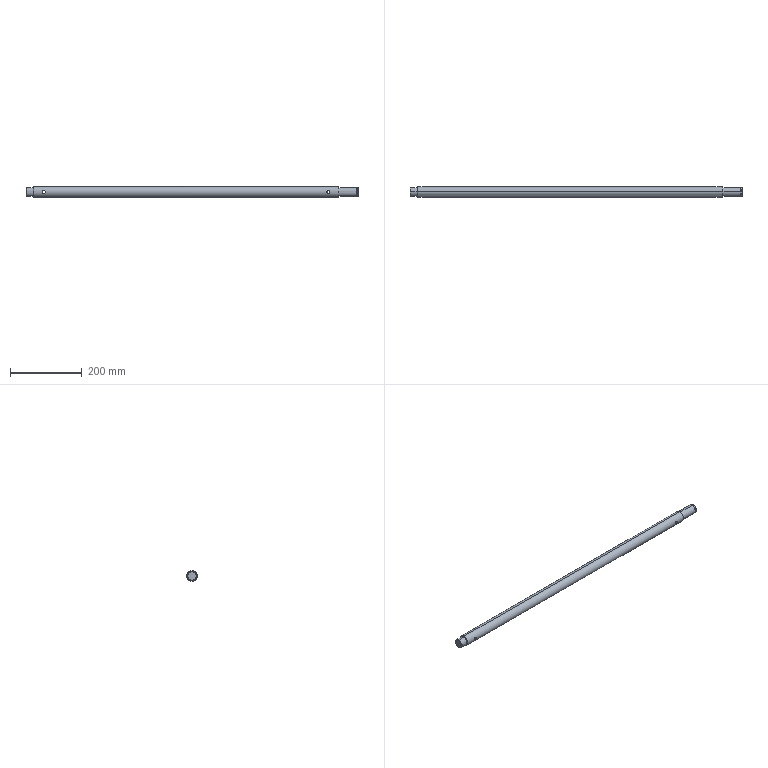Part | SolidWorks | features BaseBody 1 | 1 solid | 33 faces | box 926 x 30 x 30 mm | volume 634773 mm3 | cylinder 16 | plane 9 | cone 8 | commonest cylinder face diameters 8 x6 25 x6 23.9 x2 30 x2
STEP:
#1=CARTESIAN_POINT('',(823.,14.457,4.));
#2=VERTEX_POINT('',#1);
#3=CARTESIAN_POINT('',(823.,14.457,-4.));
#4=VERTEX_POINT('',#3);
#5=CARTESIAN_POINT('',(823.,14.457,4.));
#6=CARTESIAN_POINT('',(822.734,14.457,4.));
#7=CARTESIAN_POINT('',(822.474,14.464,3.974));
#8=CARTESIAN_POINT('',(821.961,14.492,3.871));
#9=CARTESIAN_POINT('',(821.706,14.513,3.794));
#10=CARTESIAN_POINT('',(821.222,14.564,3.593));
#11=CARTESIAN_POINT('',(820.993,14.594,3.47));
#12=CARTESIAN_POINT('',(820.559,14.66,3.18));
#13=CARTESIAN_POINT('',(820.355,14.696,3.011));
#14=CARTESIAN_POINT('',(819.987,14.766,2.644));
#15=CARTESIAN_POINT('',(819.822,14.801,2.444));
#16=CARTESIAN_POINT('',(819.53,14.867,2.007));
#17=CARTESIAN_POINT('',(819.406,14.896,1.776));
#18=CARTESIAN_POINT('',(819.206,14.946,1.295));
#19=CARTESIAN_POINT('',(819.129,14.966,1.041));
#20=CARTESIAN_POINT('',(819.026,14.993,0.5243));
#21=CARTESIAN_POINT('',(819.,15.,0.2639));
#22=CARTESIAN_POINT('',(819.,15.,-0.2606));
#23=CARTESIAN_POINT('',(819.026,14.993,-0.527));
#24=CARTESIAN_POINT('',(819.129,14.966,-1.041));
#25=CARTESIAN_POINT('',(819.205,14.946,-1.291));
#26=CARTESIAN_POINT('',(819.508,14.871,-2.02));
#27=CARTESIAN_POINT('',(819.802,14.802,-2.459));
#28=CARTESIAN_POINT('',(820.358,14.695,-3.014));
#29=CARTESIAN_POINT('',(820.558,14.66,-3.179));
#30=CARTESIAN_POINT('',(820.991,14.594,-3.469));
#31=CARTESIAN_POINT('',(821.225,14.563,-3.594));
#32=CARTESIAN_POINT('',(821.708,14.512,-3.794));
#33=CARTESIAN_POINT('',(821.957,14.492,-3.871));
#34=CARTESIAN_POINT('',(822.473,14.464,-3.974));
#35=CARTESIAN_POINT('',(822.738,14.457,-4.));
#36=CARTESIAN_POINT('',(823.,14.457,-4.));
#37=B_SPLINE_CURVE_WITH_KNOTS('',3,(#5,#6,#7,#8,#9,#10,#11,#12,#13,#14,#15,#16,#17,#18,#19,#20,#21,#22,#23,#24,#25,#26,#27,#28,#29,#30,#31,#32,#33,#34,#35,#36),.UNSPECIFIED.,.F.,.F.,(4,2,2,2,2,2,2,2,2,2,2,2,2,2,2,4),(0.,0.0007852,0.00157,0.002356,0.003141,0.003926,0.004711,0.005496,0.006281,0.007067,0.007852,0.009422,0.01021,0.01099,0.01178,0.01256),.UNSPECIFIED.);
#38=EDGE_CURVE('',#2,#4,#37,.T.);
#39=ORIENTED_EDGE('',*,*,#38,.T.);
#40=CARTESIAN_POINT('',(823.,14.457,-4.));
#41=CARTESIAN_POINT('',(823.262,14.457,-4.));
#42=CARTESIAN_POINT('',(823.523,14.464,-3.974));
#43=CARTESIAN_POINT('',(824.043,14.492,-3.871));
#44=CARTESIAN_POINT('',(824.293,14.513,-3.794));
#45=CARTESIAN_POINT('',(824.775,14.563,-3.594));
#46=CARTESIAN_POINT('',(825.009,14.594,-3.469));
#47=CARTESIAN_POINT('',(825.442,14.66,-3.179));
#48=CARTESIAN_POINT('',(825.643,14.695,-3.014));
#49=CARTESIAN_POINT('',(826.012,14.766,-2.645));
#50=CARTESIAN_POINT('',(826.18,14.802,-2.441));
#51=CARTESIAN_POINT('',(826.469,14.866,-2.009));
#52=CARTESIAN_POINT('',(826.592,14.896,-1.78));
#53=CARTESIAN_POINT('',(826.795,14.946,-1.293));
#54=CARTESIAN_POINT('',(826.871,14.966,-1.042));
#55=CARTESIAN_POINT('',(826.973,14.993,-0.5293));
#56=CARTESIAN_POINT('',(827.,15.,-0.2646));
#57=CARTESIAN_POINT('',(827.,15.,0.2628));
#58=CARTESIAN_POINT('',(826.974,14.993,0.5232));
#59=CARTESIAN_POINT('',(826.872,14.966,1.038));
#60=CARTESIAN_POINT('',(826.794,14.946,1.293));
#61=CARTESIAN_POINT('',(826.594,14.897,1.775));
#62=CARTESIAN_POINT('',(826.471,14.867,2.005));
#63=CARTESIAN_POINT('',(826.179,14.802,2.441));
#64=CARTESIAN_POINT('',(826.013,14.766,2.644));
#65=CARTESIAN_POINT('',(825.646,14.696,3.011));
#66=CARTESIAN_POINT('',(825.443,14.66,3.178));
#67=CARTESIAN_POINT('',(825.008,14.594,3.469));
#68=CARTESIAN_POINT('',(824.779,14.564,3.592));
#69=CARTESIAN_POINT('',(824.297,14.513,3.793));
#70=CARTESIAN_POINT('',(824.042,14.492,3.871));
#71=CARTESIAN_POINT('',(823.527,14.464,3.974));
#72=CARTESIAN_POINT('',(823.266,14.457,4.));
#73=CARTESIAN_POINT('',(823.,14.457,4.));
#74=B_SPLINE_CURVE_WITH_KNOTS('',3,(#40,#41,#42,#43,#44,#45,#46,#47,#48,#49,#50,#51,#52,#53,#54,#55,#56,#57,#58,#59,#60,#61,#62,#63,#64,#65,#66,#67,#68,#69,#70,#71,#72,#73),.UNSPECIFIED.,.F.,.F.,(4,2,2,2,2,2,2,2,2,2,2,2,2,2,2,2,4),(0.01256,0.01335,0.01413,0.01492,0.0157,0.01649,0.01727,0.01806,0.01884,0.01963,0.02041,0.0212,0.02198,0.02277,0.02355,0.02434,0.02512),.UNSPECIFIED.);
#75=EDGE_CURVE('',#4,#2,#74,.T.);
#76=ORIENTED_EDGE('',*,*,#75,.T.);
#77=EDGE_LOOP('',(#39,#76));
#78=FACE_BOUND('',#77,.T.);
#79=CARTESIAN_POINT('',(30.,14.457,4.));
#80=VERTEX_POINT('',#79);
#81=CARTESIAN_POINT('',(30.,14.457,-4.));
#82=VERTEX_POINT('',#81);
#83=CARTESIAN_POINT('',(30.,14.457,4.));
#84=CARTESIAN_POINT('',(29.734,14.457,4.));
#85=CARTESIAN_POINT('',(29.474,14.464,3.974));
#86=CARTESIAN_POINT('',(28.961,14.492,3.871));
#87=CARTESIAN_POINT('',(28.706,14.513,3.794));
#88=CARTESIAN_POINT('',(28.222,14.564,3.593));
#89=CARTESIAN_POINT('',(27.993,14.594,3.47));
#90=CARTESIAN_POINT('',(27.559,14.66,3.18));
#91=CARTESIAN_POINT('',(27.355,14.696,3.011));
#92=CARTESIAN_POINT('',(26.987,14.766,2.644));
#93=CARTESIAN_POINT('',(26.822,14.801,2.444));
#94=CARTESIAN_POINT('',(26.53,14.867,2.007));
#95=CARTESIAN_POINT('',(26.406,14.896,1.776));
#96=CARTESIAN_POINT('',(26.206,14.946,1.295));
#97=CARTESIAN_POINT('',(26.129,14.966,1.041));
#98=CARTESIAN_POINT('',(26.026,14.993,0.5243));
#99=CARTESIAN_POINT('',(26.,15.,0.2639));
#100=CARTESIAN_POINT('',(26.,15.,-0.2606));
#101=CARTESIAN_POINT('',(26.026,14.993,-0.527));
#102=CARTESIAN_POINT('',(26.129,14.966,-1.041));
#103=CARTESIAN_POINT('',(26.205,14.946,-1.291));
#104=CARTESIAN_POINT('',(26.508,14.871,-2.02));
#105=CARTESIAN_POINT('',(26.802,14.802,-2.459));
#106=CARTESIAN_POINT('',(27.358,14.695,-3.014));
#107=CARTESIAN_POINT('',(27.558,14.66,-3.179));
#108=CARTESIAN_POINT('',(27.991,14.594,-3.469));
#109=CARTESIAN_POINT('',(28.225,14.563,-3.594));
#110=CARTESIAN_POINT('',(28.708,14.512,-3.794));
#111=CARTESIAN_POINT('',(28.957,14.492,-3.871));
#112=CARTESIAN_POINT('',(29.473,14.464,-3.974));
#113=CARTESIAN_POINT('',(29.738,14.457,-4.));
#114=CARTESIAN_POINT('',(30.,14.457,-4.));
#115=B_SPLINE_CURVE_WITH_KNOTS('',3,(#83,#84,#85,#86,#87,#88,#89,#90,#91,#92,#93,#94,#95,#96,#97,#98,#99,#100,#101,#102,#103,#104,#105,#106,#107,#108,#109,#110,#111,#112,#113,#114),.UNSPECIFIED.,.F.,.F.,(4,2,2,2,2,2,2,2,2,2,2,2,2,2,2,4),(0.,0.0007852,0.00157,0.002356,0.003141,0.003926,0.004711,0.005496,0.006281,0.007067,0.007852,0.009422,0.01021,0.01099,0.01178,0.01256),.UNSPECIFIED.);
#116=EDGE_CURVE('',#80,#82,#115,.T.);
#117=ORIENTED_EDGE('',*,*,#116,.T.);
#118=CARTESIAN_POINT('',(30.,14.457,-4.));
#119=CARTESIAN_POINT('',(30.262,14.457,-4.));
#120=CARTESIAN_POINT('',(30.523,14.464,-3.974));
#121=CARTESIAN_POINT('',(31.043,14.492,-3.871));
#122=CARTESIAN_POINT('',(31.293,14.513,-3.794));
#123=CARTESIAN_POINT('',(31.775,14.563,-3.594));
#124=CARTESIAN_POINT('',(32.009,14.594,-3.469));
#125=CARTESIAN_POINT('',(32.442,14.66,-3.179));
#126=CARTESIAN_POINT('',(32.643,14.695,-3.014));
#127=CARTESIAN_POINT('',(33.012,14.766,-2.645));
#128=CARTESIAN_POINT('',(33.18,14.802,-2.441));
#129=CARTESIAN_POINT('',(33.469,14.866,-2.009));
#130=CARTESIAN_POINT('',(33.592,14.896,-1.78));
#131=CARTESIAN_POINT('',(33.795,14.946,-1.293));
#132=CARTESIAN_POINT('',(33.871,14.966,-1.042));
#133=CARTESIAN_POINT('',(33.973,14.993,-0.5293));
#134=CARTESIAN_POINT('',(34.,15.,-0.2646));
#135=CARTESIAN_POINT('',(34.,15.,0.2628));
#136=CARTESIAN_POINT('',(33.974,14.993,0.5232));
#137=CARTESIAN_POINT('',(33.872,14.966,1.038));
#138=CARTESIAN_POINT('',(33.794,14.946,1.293));
#139=CARTESIAN_POINT('',(33.594,14.897,1.775));
#140=CARTESIAN_POINT('',(33.471,14.867,2.005));
#141=CARTESIAN_POINT('',(33.179,14.802,2.441));
#142=CARTESIAN_POINT('',(33.013,14.766,2.644));
#143=CARTESIAN_POINT('',(32.646,14.696,3.011));
#144=CARTESIAN_POINT('',(32.443,14.66,3.178));
#145=CARTESIAN_POINT('',(32.008,14.594,3.469));
#146=CARTESIAN_POINT('',(31.779,14.564,3.592));
#147=CARTESIAN_POINT('',(31.297,14.513,3.793));
#148=CARTESIAN_POINT('',(31.042,14.492,3.871));
#149=CARTESIAN_POINT('',(30.527,14.464,3.974));
#150=CARTESIAN_POINT('',(30.266,14.457,4.));
#151=CARTESIAN_POINT('',(30.,14.457,4.));
#152=B_SPLINE_CURVE_WITH_KNOTS('',3,(#118,#119,#120,#121,#122,#123,#124,#125,#126,#127,#128,#129,#130,#131,#132,#133,#134,#135,#136,#137,#138,#139,#140,#141,#142,#143,#144,#145,#146,#147,#148,#149,#150,#151),.UNSPECIFIED.,.F.,.F.,(4,2,2,2,2,2,2,2,2,2,2,2,2,2,2,2,4),(0.01256,0.01335,0.01413,0.01492,0.0157,0.01649,0.01727,0.01806,0.01884,0.01963,0.02041,0.0212,0.02198,0.02277,0.02355,0.02434,0.02512),.UNSPECIFIED.);
#153=EDGE_CURVE('',#82,#80,#152,.T.);
#154=ORIENTED_EDGE('',*,*,#153,.T.);
#155=EDGE_LOOP('',(#117,#154));
#156=FACE_BOUND('',#155,.T.);
#157=CARTESIAN_POINT('',(1.,0.,-15.));
#158=VERTEX_POINT('',#157);
#159=CARTESIAN_POINT('',(1.,0.,15.));
#160=VERTEX_POINT('',#159);
#161=CARTESIAN_POINT('',(1.,0.,0.));
#162=DIRECTION('',(1.,0.,0.));
#163=DIRECTION('',(0.,0.,-1.));
#164=AXIS2_PLACEMENT_3D('',#161,#162,#163);
#165=CIRCLE('',#164,15.);
#166=EDGE_CURVE('',#158,#160,#165,.T.);
#167=ORIENTED_EDGE('',*,*,#166,.T.);
#168=CARTESIAN_POINT('',(852.,0.,15.));
#169=VERTEX_POINT('',#168);
#170=CARTESIAN_POINT('',(426.5,0.,15.));
#171=DIRECTION('',(1.,0.,0.));
#172=VECTOR('',#171,1000.);
#173=LINE('',#170,#172);
#174=EDGE_CURVE('',#160,#169,#173,.T.);
#175=ORIENTED_EDGE('',*,*,#174,.T.);
#176=CARTESIAN_POINT('',(852.,0.,-15.));
#177=VERTEX_POINT('',#176);
#178=CARTESIAN_POINT('',(852.,0.,0.));
#179=DIRECTION('',(-1.,0.,0.));
#180=DIRECTION('',(0.,0.,-1.));
#181=AXIS2_PLACEMENT_3D('',#178,#179,#180);
#182=CIRCLE('',#181,15.);
#183=EDGE_CURVE('',#169,#177,#182,.T.);
#184=ORIENTED_EDGE('',*,*,#183,.T.);
#185=CARTESIAN_POINT('',(426.5,0.,-15.));
#186=DIRECTION('',(1.,0.,0.));
#187=VECTOR('',#186,1000.);
#188=LINE('',#185,#187);
#189=EDGE_CURVE('',#158,#177,#188,.T.);
#190=ORIENTED_EDGE('',*,*,#189,.F.);
#191=EDGE_LOOP('',(#167,#175,#184,#190));
#192=FACE_OUTER_BOUND('',#191,.T.);
#193=CARTESIAN_POINT('',(426.5,0.,0.));
#194=DIRECTION('',(1.,0.,0.));
#195=DIRECTION('',(0.,0.,-1.));
#196=AXIS2_PLACEMENT_3D('',#193,#194,#195);
#197=CYLINDRICAL_SURFACE('',#196,15.);
#198=ADVANCED_FACE('',(#78,#156,#192),#197,.T.);
#199=CARTESIAN_POINT('',(0.,0.,-14.));
#200=VERTEX_POINT('',#199);
#201=CARTESIAN_POINT('',(0.,0.,14.));
#202=VERTEX_POINT('',#201);
#203=CARTESIAN_POINT('',(0.,0.,0.));
#204=DIRECTION('',(1.,0.,0.));
#205=DIRECTION('',(0.,0.,-1.));
#206=AXIS2_PLACEMENT_3D('',#203,#204,#205);
#207=CIRCLE('',#206,14.);
#208=EDGE_CURVE('',#200,#202,#207,.T.);
#209=ORIENTED_EDGE('',*,*,#208,.T.);
#210=CARTESIAN_POINT('',(1.,0.,15.));
#211=DIRECTION('',(0.7071,0.,0.7071));
#212=VECTOR('',#211,1000.);
#213=LINE('',#210,#212);
#214=EDGE_CURVE('',#202,#160,#213,.T.);
#215=ORIENTED_EDGE('',*,*,#214,.T.);
#216=ORIENTED_EDGE('',*,*,#166,.F.);
#217=CARTESIAN_POINT('',(1.,0.,-15.));
#218=DIRECTION('',(0.7071,0.,-0.7071));
#219=VECTOR('',#218,1000.);
#220=LINE('',#217,#219);
#221=EDGE_CURVE('',#200,#158,#220,.T.);
#222=ORIENTED_EDGE('',*,*,#221,.F.);
#223=EDGE_LOOP('',(#209,#215,#216,#222));
#224=FACE_OUTER_BOUND('',#223,.T.);
#225=CARTESIAN_POINT('',(1.,0.,0.));
#226=DIRECTION('',(1.,0.,0.));
#227=DIRECTION('',(0.,0.,-1.));
#228=AXIS2_PLACEMENT_3D('',#225,#226,#227);
#229=CONICAL_SURFACE('',#228,15.,0.7854);
#230=ADVANCED_FACE('',(#224),#229,.T.);
#231=CARTESIAN_POINT('',(30.,-14.457,-4.));
#232=VERTEX_POINT('',#231);
#233=CARTESIAN_POINT('',(30.,-14.457,4.));
#234=VERTEX_POINT('',#233);
#235=CARTESIAN_POINT('',(30.,-14.457,-4.));
#236=CARTESIAN_POINT('',(29.738,-14.457,-4.));
#237=CARTESIAN_POINT('',(29.477,-14.464,-3.974));
#238=CARTESIAN_POINT('',(28.957,-14.492,-3.871));
#239=CARTESIAN_POINT('',(28.707,-14.513,-3.794));
#240=CARTESIAN_POINT('',(28.225,-14.563,-3.594));
#241=CARTESIAN_POINT('',(27.991,-14.594,-3.469));
#242=CARTESIAN_POINT('',(27.558,-14.66,-3.179));
#243=CARTESIAN_POINT('',(27.357,-14.695,-3.014));
#244=CARTESIAN_POINT('',(26.988,-14.766,-2.645));
#245=CARTESIAN_POINT('',(26.82,-14.802,-2.441));
#246=CARTESIAN_POINT('',(26.531,-14.866,-2.009));
#247=CARTESIAN_POINT('',(26.408,-14.896,-1.78));
#248=CARTESIAN_POINT('',(26.205,-14.946,-1.293));
#249=CARTESIAN_POINT('',(26.129,-14.966,-1.042));
#250=CARTESIAN_POINT('',(26.027,-14.993,-0.5293));
#251=CARTESIAN_POINT('',(26.,-15.,-0.2646));
#252=CARTESIAN_POINT('',(26.,-15.,0.2628));
#253=CARTESIAN_POINT('',(26.026,-14.993,0.5232));
#254=CARTESIAN_POINT('',(26.128,-14.966,1.038));
#255=CARTESIAN_POINT('',(26.206,-14.946,1.293));
#256=CARTESIAN_POINT('',(26.406,-14.897,1.775));
#257=CARTESIAN_POINT('',(26.529,-14.867,2.005));
#258=CARTESIAN_POINT('',(26.821,-14.802,2.441));
#259=CARTESIAN_POINT('',(26.987,-14.766,2.644));
#260=CARTESIAN_POINT('',(27.354,-14.696,3.011));
#261=CARTESIAN_POINT('',(27.557,-14.66,3.178));
#262=CARTESIAN_POINT('',(27.992,-14.594,3.469));
#263=CARTESIAN_POINT('',(28.221,-14.564,3.592));
#264=CARTESIAN_POINT('',(28.703,-14.513,3.793));
#265=CARTESIAN_POINT('',(28.958,-14.492,3.871));
#266=CARTESIAN_POINT('',(29.473,-14.464,3.974));
#267=CARTESIAN_POINT('',(29.734,-14.457,4.));
#268=CARTESIAN_POINT('',(30.,-14.457,4.));
#269=B_SPLINE_CURVE_WITH_KNOTS('',3,(#235,#236,#237,#238,#239,#240,#241,#242,#243,#244,#245,#246,#247,#248,#249,#250,#251,#252,#253,#254,#255,#256,#257,#258,#259,#260,#261,#262,#263,#264,#265,#266,#267,#268),.UNSPECIFIED.,.F.,.F.,(4,2,2,2,2,2,2,2,2,2,2,2,2,2,2,2,4),(0.01256,0.01335,0.01413,0.01492,0.0157,0.01649,0.01727,0.01806,0.01884,0.01963,0.02041,0.0212,0.02198,0.02277,0.02355,0.02434,0.02512),.UNSPECIFIED.);
#270=EDGE_CURVE('',#232,#234,#269,.T.);
#271=ORIENTED_EDGE('',*,*,#270,.F.);
#272=CARTESIAN_POINT('',(30.,0.,-4.));
#273=DIRECTION('',(0.,1.,0.));
#274=VECTOR('',#273,1000.);
#275=LINE('',#272,#274);
#276=EDGE_CURVE('',#232,#82,#275,.T.);
#277=ORIENTED_EDGE('',*,*,#276,.T.);
#278=ORIENTED_EDGE('',*,*,#116,.F.);
#279=CARTESIAN_POINT('',(30.,0.,4.));
#280=DIRECTION('',(0.,1.,0.));
#281=VECTOR('',#280,1000.);
#282=LINE('',#279,#281);
#283=EDGE_CURVE('',#234,#80,#282,.T.);
#284=ORIENTED_EDGE('',*,*,#283,.F.);
#285=EDGE_LOOP('',(#271,#277,#278,#284));
#286=FACE_OUTER_BOUND('',#285,.T.);
#287=CARTESIAN_POINT('',(30.,0.,0.));
#288=DIRECTION('',(0.,1.,0.));
#289=DIRECTION('',(0.,0.,1.));
#290=AXIS2_PLACEMENT_3D('',#287,#288,#289);
#291=CYLINDRICAL_SURFACE('',#290,4.);
#292=ADVANCED_FACE('',(#286),#291,.F.);
#293=CARTESIAN_POINT('',(823.,-14.457,-4.));
#294=VERTEX_POINT('',#293);
#295=CARTESIAN_POINT('',(823.,-14.457,4.));
#296=VERTEX_POINT('',#295);
#297=CARTESIAN_POINT('',(823.,-14.457,-4.));
#298=CARTESIAN_POINT('',(822.738,-14.457,-4.));
#299=CARTESIAN_POINT('',(822.477,-14.464,-3.974));
#300=CARTESIAN_POINT('',(821.957,-14.492,-3.871));
#301=CARTESIAN_POINT('',(821.707,-14.513,-3.794));
#302=CARTESIAN_POINT('',(821.225,-14.563,-3.594));
#303=CARTESIAN_POINT('',(820.991,-14.594,-3.469));
#304=CARTESIAN_POINT('',(820.558,-14.66,-3.179));
#305=CARTESIAN_POINT('',(820.357,-14.695,-3.014));
#306=CARTESIAN_POINT('',(819.988,-14.766,-2.645));
#307=CARTESIAN_POINT('',(819.82,-14.802,-2.441));
#308=CARTESIAN_POINT('',(819.531,-14.866,-2.009));
#309=CARTESIAN_POINT('',(819.408,-14.896,-1.78));
#310=CARTESIAN_POINT('',(819.205,-14.946,-1.293));
#311=CARTESIAN_POINT('',(819.129,-14.966,-1.042));
#312=CARTESIAN_POINT('',(819.027,-14.993,-0.5293));
#313=CARTESIAN_POINT('',(819.,-15.,-0.2646));
#314=CARTESIAN_POINT('',(819.,-15.,0.2628));
#315=CARTESIAN_POINT('',(819.026,-14.993,0.5232));
#316=CARTESIAN_POINT('',(819.128,-14.966,1.038));
#317=CARTESIAN_POINT('',(819.206,-14.946,1.293));
#318=CARTESIAN_POINT('',(819.406,-14.897,1.775));
#319=CARTESIAN_POINT('',(819.529,-14.867,2.005));
#320=CARTESIAN_POINT('',(819.821,-14.802,2.441));
#321=CARTESIAN_POINT('',(819.987,-14.766,2.644));
#322=CARTESIAN_POINT('',(820.354,-14.696,3.011));
#323=CARTESIAN_POINT('',(820.557,-14.66,3.178));
#324=CARTESIAN_POINT('',(820.992,-14.594,3.469));
#325=CARTESIAN_POINT('',(821.221,-14.564,3.592));
#326=CARTESIAN_POINT('',(821.703,-14.513,3.793));
#327=CARTESIAN_POINT('',(821.958,-14.492,3.871));
#328=CARTESIAN_POINT('',(822.473,-14.464,3.974));
#329=CARTESIAN_POINT('',(822.734,-14.457,4.));
#330=CARTESIAN_POINT('',(823.,-14.457,4.));
#331=B_SPLINE_CURVE_WITH_KNOTS('',3,(#297,#298,#299,#300,#301,#302,#303,#304,#305,#306,#307,#308,#309,#310,#311,#312,#313,#314,#315,#316,#317,#318,#319,#320,#321,#322,#323,#324,#325,#326,#327,#328,#329,#330),.UNSPECIFIED.,.F.,.F.,(4,2,2,2,2,2,2,2,2,2,2,2,2,2,2,2,4),(0.01256,0.01335,0.01413,0.01492,0.0157,0.01649,0.01727,0.01806,0.01884,0.01963,0.02041,0.0212,0.02198,0.02277,0.02355,0.02434,0.02512),.UNSPECIFIED.);
#332=EDGE_CURVE('',#294,#296,#331,.T.);
#333=ORIENTED_EDGE('',*,*,#332,.F.);
#334=CARTESIAN_POINT('',(823.,0.,-4.));
#335=DIRECTION('',(0.,1.,0.));
#336=VECTOR('',#335,1000.);
#337=LINE('',#334,#336);
#338=EDGE_CURVE('',#294,#4,#337,.T.);
#339=ORIENTED_EDGE('',*,*,#338,.T.);
#340=ORIENTED_EDGE('',*,*,#38,.F.);
#341=CARTESIAN_POINT('',(823.,0.,4.));
#342=DIRECTION('',(0.,1.,0.));
#343=VECTOR('',#342,1000.);
#344=LINE('',#341,#343);
#345=EDGE_CURVE('',#296,#2,#344,.T.);
#346=ORIENTED_EDGE('',*,*,#345,.F.);
#347=EDGE_LOOP('',(#333,#339,#340,#346));
#348=FACE_OUTER_BOUND('',#347,.T.);
#349=CARTESIAN_POINT('',(823.,0.,0.));
#350=DIRECTION('',(0.,1.,0.));
#351=DIRECTION('',(0.,0.,1.));
#352=AXIS2_PLACEMENT_3D('',#349,#350,#351);
#353=CYLINDRICAL_SURFACE('',#352,4.);
#354=ADVANCED_FACE('',(#348),#353,.F.);
#355=CARTESIAN_POINT('',(853.,0.,14.));
#356=VERTEX_POINT('',#355);
#357=CARTESIAN_POINT('',(853.,0.,-14.));
#358=VERTEX_POINT('',#357);
#359=CARTESIAN_POINT('',(853.,0.,0.));
#360=DIRECTION('',(-1.,0.,0.));
#361=DIRECTION('',(0.,0.,1.));
#362=AXIS2_PLACEMENT_3D('',#359,#360,#361);
#363=CIRCLE('',#362,14.);
#364=EDGE_CURVE('',#356,#358,#363,.T.);
#365=ORIENTED_EDGE('',*,*,#364,.T.);
#366=CARTESIAN_POINT('',(852.,0.,-15.));
#367=DIRECTION('',(-0.7071,0.,-0.7071));
#368=VECTOR('',#367,1000.);
#369=LINE('',#366,#368);
#370=EDGE_CURVE('',#358,#177,#369,.T.);
#371=ORIENTED_EDGE('',*,*,#370,.T.);
#372=ORIENTED_EDGE('',*,*,#183,.F.);
#373=CARTESIAN_POINT('',(852.,0.,15.));
#374=DIRECTION('',(-0.7071,0.,0.7071));
#375=VECTOR('',#374,1000.);
#376=LINE('',#373,#375);
#377=EDGE_CURVE('',#356,#169,#376,.T.);
#378=ORIENTED_EDGE('',*,*,#377,.F.);
#379=EDGE_LOOP('',(#365,#371,#372,#378));
#380=FACE_OUTER_BOUND('',#379,.T.);
#381=CARTESIAN_POINT('',(852.,0.,0.));
#382=DIRECTION('',(-1.,0.,0.));
#383=DIRECTION('',(0.,0.,1.));
#384=AXIS2_PLACEMENT_3D('',#381,#382,#383);
#385=CONICAL_SURFACE('',#384,15.,0.7854);
#386=ADVANCED_FACE('',(#380),#385,.T.);
#387=CARTESIAN_POINT('',(-19.,0.,-12.5));
#388=VERTEX_POINT('',#387);
#389=CARTESIAN_POINT('',(-19.,0.,12.5));
#390=VERTEX_POINT('',#389);
#391=CARTESIAN_POINT('',(-19.,0.,0.));
#392=DIRECTION('',(1.,0.,0.));
#393=DIRECTION('',(0.,0.,-1.));
#394=AXIS2_PLACEMENT_3D('',#391,#392,#393);
#395=CIRCLE('',#394,12.5);
#396=EDGE_CURVE('',#388,#390,#395,.T.);
#397=ORIENTED_EDGE('',*,*,#396,.T.);
#398=CARTESIAN_POINT('',(0.,0.,12.5));
#399=VERTEX_POINT('',#398);
#400=CARTESIAN_POINT('',(-10.,0.,12.5));
#401=DIRECTION('',(1.,0.,0.));
#402=VECTOR('',#401,1000.);
#403=LINE('',#400,#402);
#404=EDGE_CURVE('',#390,#399,#403,.T.);
#405=ORIENTED_EDGE('',*,*,#404,.T.);
#406=CARTESIAN_POINT('',(0.,0.,-12.5));
#407=VERTEX_POINT('',#406);
#408=CARTESIAN_POINT('',(0.,0.,0.));
#409=DIRECTION('',(1.,0.,0.));
#410=DIRECTION('',(0.,0.,-1.));
#411=AXIS2_PLACEMENT_3D('',#408,#409,#410);
#412=CIRCLE('',#411,12.5);
#413=EDGE_CURVE('',#407,#399,#412,.T.);
#414=ORIENTED_EDGE('',*,*,#413,.F.);
#415=CARTESIAN_POINT('',(-10.,0.,-12.5));
#416=DIRECTION('',(1.,0.,0.));
#417=VECTOR('',#416,1000.);
#418=LINE('',#415,#417);
#419=EDGE_CURVE('',#388,#407,#418,.T.);
#420=ORIENTED_EDGE('',*,*,#419,.F.);
#421=EDGE_LOOP('',(#397,#405,#414,#420));
#422=FACE_OUTER_BOUND('',#421,.T.);
#423=CARTESIAN_POINT('',(-10.,0.,0.));
#424=DIRECTION('',(1.,0.,0.));
#425=DIRECTION('',(0.,0.,-1.));
#426=AXIS2_PLACEMENT_3D('',#423,#424,#425);
#427=CYLINDRICAL_SURFACE('',#426,12.5);
#428=ADVANCED_FACE('',(#422),#427,.T.);
#429=CARTESIAN_POINT('',(874.,11.843,4.));
#430=VERTEX_POINT('',#429);
#431=CARTESIAN_POINT('',(874.,11.843,-4.));
#432=VERTEX_POINT('',#431);
#433=CARTESIAN_POINT('',(874.,11.843,4.));
#434=CARTESIAN_POINT('',(873.734,11.843,4.));
#435=CARTESIAN_POINT('',(873.473,11.852,3.974));
#436=CARTESIAN_POINT('',(872.959,11.886,3.871));
#437=CARTESIAN_POINT('',(872.705,11.911,3.794));
#438=CARTESIAN_POINT('',(872.221,11.973,3.592));
#439=CARTESIAN_POINT('',(871.993,12.01,3.47));
#440=CARTESIAN_POINT('',(871.559,12.09,3.18));
#441=CARTESIAN_POINT('',(871.356,12.133,3.012));
#442=CARTESIAN_POINT('',(870.989,12.218,2.646));
#443=CARTESIAN_POINT('',(870.824,12.26,2.446));
#444=CARTESIAN_POINT('',(870.532,12.339,2.01));
#445=CARTESIAN_POINT('',(870.409,12.375,1.78));
#446=CARTESIAN_POINT('',(870.208,12.435,1.3));
#447=CARTESIAN_POINT('',(870.13,12.459,1.047));
#448=CARTESIAN_POINT('',(870.026,12.492,0.5284));
#449=CARTESIAN_POINT('',(870.,12.5,0.266));
#450=CARTESIAN_POINT('',(870.,12.5,-0.266));
#451=CARTESIAN_POINT('',(870.026,12.492,-0.5273));
#452=CARTESIAN_POINT('',(870.129,12.459,-1.041));
#453=CARTESIAN_POINT('',(870.207,12.435,-1.296));
#454=CARTESIAN_POINT('',(870.408,12.375,-1.779));
#455=CARTESIAN_POINT('',(870.531,12.34,-2.008));
#456=CARTESIAN_POINT('',(870.821,12.261,-2.441));
#457=CARTESIAN_POINT('',(870.988,12.218,-2.645));
#458=CARTESIAN_POINT('',(871.354,12.133,-3.011));
#459=CARTESIAN_POINT('',(871.554,12.091,-3.176));
#460=CARTESIAN_POINT('',(871.991,12.01,-3.469));
#461=CARTESIAN_POINT('',(872.22,11.973,-3.592));
#462=CARTESIAN_POINT('',(872.7,11.911,-3.792));
#463=CARTESIAN_POINT('',(872.954,11.886,-3.87));
#464=CARTESIAN_POINT('',(873.472,11.852,-3.974));
#465=CARTESIAN_POINT('',(873.734,11.843,-4.));
#466=CARTESIAN_POINT('',(874.,11.843,-4.));
#467=B_SPLINE_CURVE_WITH_KNOTS('',3,(#433,#434,#435,#436,#437,#438,#439,#440,#441,#442,#443,#444,#445,#446,#447,#448,#449,#450,#451,#452,#453,#454,#455,#456,#457,#458,#459,#460,#461,#462,#463,#464,#465,#466),.UNSPECIFIED.,.F.,.F.,(4,2,2,2,2,2,2,2,2,2,2,2,2,2,2,2,4),(-0.00629,-0.005504,-0.004718,-0.003931,-0.003145,-0.002359,-0.001573,-0.0007863,0.000000038,0.0007863,0.001573,0.002359,0.003145,0.003932,0.004718,0.005504,0.00629),.UNSPECIFIED.);
#468=EDGE_CURVE('',#430,#432,#467,.T.);
#469=ORIENTED_EDGE('',*,*,#468,.T.);
#470=CARTESIAN_POINT('',(894.,11.843,-4.));
#471=VERTEX_POINT('',#470);
#472=CARTESIAN_POINT('',(877.,11.843,-4.));
#473=DIRECTION('',(1.,0.,0.));
#474=VECTOR('',#473,1000.);
#475=LINE('',#472,#474);
#476=EDGE_CURVE('',#432,#471,#475,.T.);
#477=ORIENTED_EDGE('',*,*,#476,.T.);
#478=CARTESIAN_POINT('',(894.,11.843,4.));
#479=VERTEX_POINT('',#478);
#480=CARTESIAN_POINT('',(894.,11.843,-4.));
#481=CARTESIAN_POINT('',(894.266,11.843,-4.));
#482=CARTESIAN_POINT('',(894.527,11.852,-3.974));
#483=CARTESIAN_POINT('',(895.041,11.886,-3.871));
#484=CARTESIAN_POINT('',(895.295,11.911,-3.794));
#485=CARTESIAN_POINT('',(895.779,11.973,-3.592));
#486=CARTESIAN_POINT('',(896.007,12.01,-3.47));
#487=CARTESIAN_POINT('',(896.441,12.09,-3.18));
#488=CARTESIAN_POINT('',(896.644,12.133,-3.012));
#489=CARTESIAN_POINT('',(897.011,12.218,-2.646));
#490=CARTESIAN_POINT('',(897.176,12.26,-2.446));
#491=CARTESIAN_POINT('',(897.468,12.339,-2.01));
#492=CARTESIAN_POINT('',(897.591,12.375,-1.78));
#493=CARTESIAN_POINT('',(897.792,12.435,-1.3));
#494=CARTESIAN_POINT('',(897.87,12.459,-1.047));
#495=CARTESIAN_POINT('',(897.974,12.492,-0.5284));
#496=CARTESIAN_POINT('',(898.,12.5,-0.266));
#497=CARTESIAN_POINT('',(898.,12.5,0.266));
#498=CARTESIAN_POINT('',(897.974,12.492,0.5273));
#499=CARTESIAN_POINT('',(897.871,12.459,1.041));
#500=CARTESIAN_POINT('',(897.793,12.435,1.296));
#501=CARTESIAN_POINT('',(897.592,12.375,1.779));
#502=CARTESIAN_POINT('',(897.469,12.34,2.008));
#503=CARTESIAN_POINT('',(897.179,12.261,2.441));
#504=CARTESIAN_POINT('',(897.012,12.218,2.645));
#505=CARTESIAN_POINT('',(896.646,12.133,3.011));
#506=CARTESIAN_POINT('',(896.446,12.091,3.176));
#507=CARTESIAN_POINT('',(896.009,12.01,3.469));
#508=CARTESIAN_POINT('',(895.78,11.973,3.592));
#509=CARTESIAN_POINT('',(895.3,11.911,3.792));
#510=CARTESIAN_POINT('',(895.046,11.886,3.87));
#511=CARTESIAN_POINT('',(894.528,11.852,3.974));
#512=CARTESIAN_POINT('',(894.266,11.843,4.));
#513=CARTESIAN_POINT('',(894.,11.843,4.));
#514=B_SPLINE_CURVE_WITH_KNOTS('',3,(#480,#481,#482,#483,#484,#485,#486,#487,#488,#489,#490,#491,#492,#493,#494,#495,#496,#497,#498,#499,#500,#501,#502,#503,#504,#505,#506,#507,#508,#509,#510,#511,#512,#513),.UNSPECIFIED.,.F.,.F.,(4,2,2,2,2,2,2,2,2,2,2,2,2,2,2,2,4),(-0.00629,-0.005504,-0.004718,-0.003931,-0.003145,-0.002359,-0.001573,-0.0007863,0.000000038,0.0007863,0.001573,0.002359,0.003145,0.003932,0.004718,0.005504,0.00629),.UNSPECIFIED.);
#515=EDGE_CURVE('',#471,#479,#514,.T.);
#516=ORIENTED_EDGE('',*,*,#515,.T.);
#517=CARTESIAN_POINT('',(877.,11.843,4.));
#518=DIRECTION('',(-1.,0.,0.));
#519=VECTOR('',#518,1000.);
#520=LINE('',#517,#519);
#521=EDGE_CURVE('',#479,#430,#520,.T.);
#522=ORIENTED_EDGE('',*,*,#521,.T.);
#523=EDGE_LOOP('',(#469,#477,#516,#522));
#524=FACE_BOUND('',#523,.T.);
#525=CARTESIAN_POINT('',(853.,0.,12.5));
#526=VERTEX_POINT('',#525);
#527=CARTESIAN_POINT('',(853.,0.,-12.5));
#528=VERTEX_POINT('',#527);
#529=CARTESIAN_POINT('',(853.,0.,0.));
#530=DIRECTION('',(-1.,0.,0.));
#531=DIRECTION('',(0.,0.,-1.));
#532=AXIS2_PLACEMENT_3D('',#529,#530,#531);
#533=CIRCLE('',#532,12.5);
#534=EDGE_CURVE('',#526,#528,#533,.T.);
#535=ORIENTED_EDGE('',*,*,#534,.F.);
#536=CARTESIAN_POINT('',(901.,0.,12.5));
#537=VERTEX_POINT('',#536);
#538=CARTESIAN_POINT('',(877.,0.,12.5));
#539=DIRECTION('',(1.,0.,0.));
#540=VECTOR('',#539,1000.);
#541=LINE('',#538,#540);
#542=EDGE_CURVE('',#526,#537,#541,.T.);
#543=ORIENTED_EDGE('',*,*,#542,.T.);
#544=CARTESIAN_POINT('',(901.,0.,-12.5));
#545=VERTEX_POINT('',#544);
#546=CARTESIAN_POINT('',(901.,0.,0.));
#547=DIRECTION('',(-1.,0.,0.));
#548=DIRECTION('',(0.,0.,-1.));
#549=AXIS2_PLACEMENT_3D('',#546,#547,#548);
#550=CIRCLE('',#549,12.5);
#551=EDGE_CURVE('',#537,#545,#550,.T.);
#552=ORIENTED_EDGE('',*,*,#551,.T.);
#553=CARTESIAN_POINT('',(877.,0.,-12.5));
#554=DIRECTION('',(1.,0.,0.));
#555=VECTOR('',#554,1000.);
#556=LINE('',#553,#555);
#557=EDGE_CURVE('',#528,#545,#556,.T.);
#558=ORIENTED_EDGE('',*,*,#557,.F.);
#559=EDGE_LOOP('',(#535,#543,#552,#558));
#560=FACE_OUTER_BOUND('',#559,.T.);
#561=CARTESIAN_POINT('',(877.,0.,0.));
#562=DIRECTION('',(1.,0.,0.));
#563=DIRECTION('',(0.,0.,-1.));
#564=AXIS2_PLACEMENT_3D('',#561,#562,#563);
#565=CYLINDRICAL_SURFACE('',#564,12.5);
#566=ADVANCED_FACE('',(#524,#560),#565,.T.);
#567=CARTESIAN_POINT('',(-20.,0.,-11.5));
#568=VERTEX_POINT('',#567);
#569=CARTESIAN_POINT('',(-20.,0.,11.5));
#570=VERTEX_POINT('',#569);
#571=CARTESIAN_POINT('',(-20.,0.,0.));
#572=DIRECTION('',(1.,0.,0.));
#573=DIRECTION('',(0.,0.,-1.));
#574=AXIS2_PLACEMENT_3D('',#571,#572,#573);
#575=CIRCLE('',#574,11.5);
#576=EDGE_CURVE('',#568,#570,#575,.T.);
#577=ORIENTED_EDGE('',*,*,#576,.T.);
#578=CARTESIAN_POINT('',(-19.,0.,12.5));
#579=DIRECTION('',(0.7071,0.,0.7071));
#580=VECTOR('',#579,1000.);
#581=LINE('',#578,#580);
#582=EDGE_CURVE('',#570,#390,#581,.T.);
#583=ORIENTED_EDGE('',*,*,#582,.T.);
#584=ORIENTED_EDGE('',*,*,#396,.F.);
#585=CARTESIAN_POINT('',(-19.,0.,-12.5));
#586=DIRECTION('',(0.7071,0.,-0.7071));
#587=VECTOR('',#586,1000.);
#588=LINE('',#585,#587);
#589=EDGE_CURVE('',#568,#388,#588,.T.);
#590=ORIENTED_EDGE('',*,*,#589,.F.);
#591=EDGE_LOOP('',(#577,#583,#584,#590));
#592=FACE_OUTER_BOUND('',#591,.T.);
#593=CARTESIAN_POINT('',(-19.,0.,0.));
#594=DIRECTION('',(1.,0.,0.));
#595=DIRECTION('',(0.,0.,-1.));
#596=AXIS2_PLACEMENT_3D('',#593,#594,#595);
#597=CONICAL_SURFACE('',#596,12.5,0.7854);
#598=ADVANCED_FACE('',(#592),#597,.T.);
#599=CARTESIAN_POINT('',(901.,0.,11.95));
#600=VERTEX_POINT('',#599);
#601=CARTESIAN_POINT('',(901.,0.,-11.95));
#602=VERTEX_POINT('',#601);
#603=CARTESIAN_POINT('',(901.,0.,0.));
#604=DIRECTION('',(-1.,0.,0.));
#605=DIRECTION('',(0.,0.,-1.));
#606=AXIS2_PLACEMENT_3D('',#603,#604,#605);
#607=CIRCLE('',#606,11.95);
#608=EDGE_CURVE('',#600,#602,#607,.T.);
#609=ORIENTED_EDGE('',*,*,#608,.F.);
#610=CARTESIAN_POINT('',(902.3,0.,11.95));
#611=VERTEX_POINT('',#610);
#612=CARTESIAN_POINT('',(901.65,0.,11.95));
#613=DIRECTION('',(1.,0.,0.));
#614=VECTOR('',#613,1000.);
#615=LINE('',#612,#614);
#616=EDGE_CURVE('',#600,#611,#615,.T.);
#617=ORIENTED_EDGE('',*,*,#616,.T.);
#618=CARTESIAN_POINT('',(902.3,0.,-11.95));
#619=VERTEX_POINT('',#618);
#620=CARTESIAN_POINT('',(902.3,0.,0.));
#621=DIRECTION('',(-1.,0.,0.));
#622=DIRECTION('',(0.,0.,-1.));
#623=AXIS2_PLACEMENT_3D('',#620,#621,#622);
#624=CIRCLE('',#623,11.95);
#625=EDGE_CURVE('',#611,#619,#624,.T.);
#626=ORIENTED_EDGE('',*,*,#625,.T.);
#627=CARTESIAN_POINT('',(901.65,0.,-11.95));
#628=DIRECTION('',(1.,0.,0.));
#629=VECTOR('',#628,1000.);
#630=LINE('',#627,#629);
#631=EDGE_CURVE('',#602,#619,#630,.T.);
#632=ORIENTED_EDGE('',*,*,#631,.F.);
#633=EDGE_LOOP('',(#609,#617,#626,#632));
#634=FACE_OUTER_BOUND('',#633,.T.);
#635=CARTESIAN_POINT('',(901.65,0.,0.));
#636=DIRECTION('',(1.,0.,0.));
#637=DIRECTION('',(0.,0.,-1.));
#638=AXIS2_PLACEMENT_3D('',#635,#636,#637);
#639=CYLINDRICAL_SURFACE('',#638,11.95);
#640=ADVANCED_FACE('',(#634),#639,.T.);
#641=CARTESIAN_POINT('',(902.3,0.,12.5));
#642=VERTEX_POINT('',#641);
#643=CARTESIAN_POINT('',(902.3,0.,-12.5));
#644=VERTEX_POINT('',#643);
#645=CARTESIAN_POINT('',(902.3,0.,0.));
#646=DIRECTION('',(-1.,0.,0.));
#647=DIRECTION('',(0.,0.,-1.));
#648=AXIS2_PLACEMENT_3D('',#645,#646,#647);
#649=CIRCLE('',#648,12.5);
#650=EDGE_CURVE('',#642,#644,#649,.T.);
#651=ORIENTED_EDGE('',*,*,#650,.F.);
#652=CARTESIAN_POINT('',(905.,0.,12.5));
#653=VERTEX_POINT('',#652);
#654=CARTESIAN_POINT('',(904.15,0.,12.5));
#655=DIRECTION('',(1.,0.,0.));
#656=VECTOR('',#655,1000.);
#657=LINE('',#654,#656);
#658=EDGE_CURVE('',#642,#653,#657,.T.);
#659=ORIENTED_EDGE('',*,*,#658,.T.);
#660=CARTESIAN_POINT('',(905.,0.,-12.5));
#661=VERTEX_POINT('',#660);
#662=CARTESIAN_POINT('',(905.,0.,0.));
#663=DIRECTION('',(-1.,0.,0.));
#664=DIRECTION('',(0.,0.,-1.));
#665=AXIS2_PLACEMENT_3D('',#662,#663,#664);
#666=CIRCLE('',#665,12.5);
#667=EDGE_CURVE('',#653,#661,#666,.T.);
#668=ORIENTED_EDGE('',*,*,#667,.T.);
#669=CARTESIAN_POINT('',(904.15,0.,-12.5));
#670=DIRECTION('',(1.,0.,0.));
#671=VECTOR('',#670,1000.);
#672=LINE('',#669,#671);
#673=EDGE_CURVE('',#644,#661,#672,.T.);
#674=ORIENTED_EDGE('',*,*,#673,.F.);
#675=EDGE_LOOP('',(#651,#659,#668,#674));
#676=FACE_OUTER_BOUND('',#675,.T.);
#677=CARTESIAN_POINT('',(904.15,0.,0.));
#678=DIRECTION('',(1.,0.,0.));
#679=DIRECTION('',(0.,0.,-1.));
#680=AXIS2_PLACEMENT_3D('',#677,#678,#679);
#681=CYLINDRICAL_SURFACE('',#680,12.5);
#682=ADVANCED_FACE('',(#676),#681,.T.);
#683=CARTESIAN_POINT('',(906.,0.,11.5));
#684=VERTEX_POINT('',#683);
#685=CARTESIAN_POINT('',(906.,0.,-11.5));
#686=VERTEX_POINT('',#685);
#687=CARTESIAN_POINT('',(906.,0.,0.));
#688=DIRECTION('',(-1.,0.,0.));
#689=DIRECTION('',(0.,0.,1.));
#690=AXIS2_PLACEMENT_3D('',#687,#688,#689);
#691=CIRCLE('',#690,11.5);
#692=EDGE_CURVE('',#684,#686,#691,.T.);
#693=ORIENTED_EDGE('',*,*,#692,.T.);
#694=CARTESIAN_POINT('',(905.,0.,-12.5));
#695=DIRECTION('',(-0.7071,0.,-0.7071));
#696=VECTOR('',#695,1000.);
#697=LINE('',#694,#696);
#698=EDGE_CURVE('',#686,#661,#697,.T.);
#699=ORIENTED_EDGE('',*,*,#698,.T.);
#700=ORIENTED_EDGE('',*,*,#667,.F.);
#701=CARTESIAN_POINT('',(905.,0.,12.5));
#702=DIRECTION('',(-0.7071,0.,0.7071));
#703=VECTOR('',#702,1000.);
#704=LINE('',#701,#703);
#705=EDGE_CURVE('',#684,#653,#704,.T.);
#706=ORIENTED_EDGE('',*,*,#705,.F.);
#707=EDGE_LOOP('',(#693,#699,#700,#706));
#708=FACE_OUTER_BOUND('',#707,.T.);
#709=CARTESIAN_POINT('',(905.,0.,0.));
#710=DIRECTION('',(-1.,0.,0.));
#711=DIRECTION('',(0.,0.,1.));
#712=AXIS2_PLACEMENT_3D('',#709,#710,#711);
#713=CONICAL_SURFACE('',#712,12.5,0.7854);
#714=ADVANCED_FACE('',(#708),#713,.T.);
#715=ORIENTED_EDGE('',*,*,#174,.F.);
#716=CARTESIAN_POINT('',(1.,0.,0.));
#717=DIRECTION('',(1.,0.,0.));
#718=DIRECTION('',(0.,0.,-1.));
#719=AXIS2_PLACEMENT_3D('',#716,#717,#718);
#720=CIRCLE('',#719,15.);
#721=EDGE_CURVE('',#160,#158,#720,.T.);
#722=ORIENTED_EDGE('',*,*,#721,.T.);
#723=ORIENTED_EDGE('',*,*,#189,.T.);
#724=CARTESIAN_POINT('',(852.,0.,0.));
#725=DIRECTION('',(-1.,0.,0.));
#726=DIRECTION('',(0.,0.,-1.));
#727=AXIS2_PLACEMENT_3D('',#724,#725,#726);
#728=CIRCLE('',#727,15.);
#729=EDGE_CURVE('',#177,#169,#728,.T.);
#730=ORIENTED_EDGE('',*,*,#729,.T.);
#731=EDGE_LOOP('',(#715,#722,#723,#730));
#732=FACE_OUTER_BOUND('',#731,.T.);
#733=CARTESIAN_POINT('',(30.,-14.457,4.));
#734=CARTESIAN_POINT('',(30.266,-14.457,4.));
#735=CARTESIAN_POINT('',(30.526,-14.464,3.974));
#736=CARTESIAN_POINT('',(31.039,-14.492,3.871));
#737=CARTESIAN_POINT('',(31.294,-14.513,3.794));
#738=CARTESIAN_POINT('',(31.778,-14.564,3.593));
#739=CARTESIAN_POINT('',(32.007,-14.594,3.47));
#740=CARTESIAN_POINT('',(32.441,-14.66,3.18));
#741=CARTESIAN_POINT('',(32.645,-14.696,3.011));
#742=CARTESIAN_POINT('',(33.013,-14.766,2.644));
#743=CARTESIAN_POINT('',(33.178,-14.801,2.444));
#744=CARTESIAN_POINT('',(33.47,-14.867,2.007));
#745=CARTESIAN_POINT('',(33.594,-14.896,1.776));
#746=CARTESIAN_POINT('',(33.794,-14.946,1.295));
#747=CARTESIAN_POINT('',(33.871,-14.966,1.041));
#748=CARTESIAN_POINT('',(33.974,-14.993,0.5243));
#749=CARTESIAN_POINT('',(34.,-15.,0.2639));
#750=CARTESIAN_POINT('',(34.,-15.,-0.2606));
#751=CARTESIAN_POINT('',(33.974,-14.993,-0.527));
#752=CARTESIAN_POINT('',(33.871,-14.966,-1.041));
#753=CARTESIAN_POINT('',(33.795,-14.946,-1.291));
#754=CARTESIAN_POINT('',(33.492,-14.871,-2.02));
#755=CARTESIAN_POINT('',(33.198,-14.802,-2.459));
#756=CARTESIAN_POINT('',(32.642,-14.695,-3.014));
#757=CARTESIAN_POINT('',(32.442,-14.66,-3.179));
#758=CARTESIAN_POINT('',(32.009,-14.594,-3.469));
#759=CARTESIAN_POINT('',(31.775,-14.563,-3.594));
#760=CARTESIAN_POINT('',(31.292,-14.512,-3.794));
#761=CARTESIAN_POINT('',(31.043,-14.492,-3.871));
#762=CARTESIAN_POINT('',(30.527,-14.464,-3.974));
#763=CARTESIAN_POINT('',(30.262,-14.457,-4.));
#764=CARTESIAN_POINT('',(30.,-14.457,-4.));
#765=B_SPLINE_CURVE_WITH_KNOTS('',3,(#733,#734,#735,#736,#737,#738,#739,#740,#741,#742,#743,#744,#745,#746,#747,#748,#749,#750,#751,#752,#753,#754,#755,#756,#757,#758,#759,#760,#761,#762,#763,#764),.UNSPECIFIED.,.F.,.F.,(4,2,2,2,2,2,2,2,2,2,2,2,2,2,2,4),(0.,0.0007852,0.00157,0.002356,0.003141,0.003926,0.004711,0.005496,0.006281,0.007067,0.007852,0.009422,0.01021,0.01099,0.01178,0.01256),.UNSPECIFIED.);
#766=EDGE_CURVE('',#234,#232,#765,.T.);
#767=ORIENTED_EDGE('',*,*,#766,.T.);
#768=ORIENTED_EDGE('',*,*,#270,.T.);
#769=EDGE_LOOP('',(#767,#768));
#770=FACE_BOUND('',#769,.T.);
#771=CARTESIAN_POINT('',(823.,-14.457,4.));
#772=CARTESIAN_POINT('',(823.266,-14.457,4.));
#773=CARTESIAN_POINT('',(823.526,-14.464,3.974));
#774=CARTESIAN_POINT('',(824.039,-14.492,3.871));
#775=CARTESIAN_POINT('',(824.294,-14.513,3.794));
#776=CARTESIAN_POINT('',(824.778,-14.564,3.593));
#777=CARTESIAN_POINT('',(825.007,-14.594,3.47));
#778=CARTESIAN_POINT('',(825.441,-14.66,3.18));
#779=CARTESIAN_POINT('',(825.645,-14.696,3.011));
#780=CARTESIAN_POINT('',(826.013,-14.766,2.644));
#781=CARTESIAN_POINT('',(826.178,-14.801,2.444));
#782=CARTESIAN_POINT('',(826.47,-14.867,2.007));
#783=CARTESIAN_POINT('',(826.594,-14.896,1.776));
#784=CARTESIAN_POINT('',(826.794,-14.946,1.295));
#785=CARTESIAN_POINT('',(826.871,-14.966,1.041));
#786=CARTESIAN_POINT('',(826.974,-14.993,0.5243));
#787=CARTESIAN_POINT('',(827.,-15.,0.2639));
#788=CARTESIAN_POINT('',(827.,-15.,-0.2606));
#789=CARTESIAN_POINT('',(826.974,-14.993,-0.527));
#790=CARTESIAN_POINT('',(826.871,-14.966,-1.041));
#791=CARTESIAN_POINT('',(826.795,-14.946,-1.291));
#792=CARTESIAN_POINT('',(826.492,-14.871,-2.02));
#793=CARTESIAN_POINT('',(826.198,-14.802,-2.459));
#794=CARTESIAN_POINT('',(825.642,-14.695,-3.014));
#795=CARTESIAN_POINT('',(825.442,-14.66,-3.179));
#796=CARTESIAN_POINT('',(825.009,-14.594,-3.469));
#797=CARTESIAN_POINT('',(824.775,-14.563,-3.594));
#798=CARTESIAN_POINT('',(824.292,-14.512,-3.794));
#799=CARTESIAN_POINT('',(824.043,-14.492,-3.871));
#800=CARTESIAN_POINT('',(823.527,-14.464,-3.974));
#801=CARTESIAN_POINT('',(823.262,-14.457,-4.));
#802=CARTESIAN_POINT('',(823.,-14.457,-4.));
#803=B_SPLINE_CURVE_WITH_KNOTS('',3,(#771,#772,#773,#774,#775,#776,#777,#778,#779,#780,#781,#782,#783,#784,#785,#786,#787,#788,#789,#790,#791,#792,#793,#794,#795,#796,#797,#798,#799,#800,#801,#802),.UNSPECIFIED.,.F.,.F.,(4,2,2,2,2,2,2,2,2,2,2,2,2,2,2,4),(0.,0.0007852,0.00157,0.002356,0.003141,0.003926,0.004711,0.005496,0.006281,0.007067,0.007852,0.009422,0.01021,0.01099,0.01178,0.01256),.UNSPECIFIED.);
#804=EDGE_CURVE('',#296,#294,#803,.T.);
#805=ORIENTED_EDGE('',*,*,#804,.T.);
#806=ORIENTED_EDGE('',*,*,#332,.T.);
#807=EDGE_LOOP('',(#805,#806));
#808=FACE_BOUND('',#807,.T.);
#809=CARTESIAN_POINT('',(426.5,0.,0.));
#810=DIRECTION('',(1.,0.,0.));
#811=DIRECTION('',(0.,0.,-1.));
#812=AXIS2_PLACEMENT_3D('',#809,#810,#811);
#813=CYLINDRICAL_SURFACE('',#812,15.);
#814=ADVANCED_FACE('',(#732,#770,#808),#813,.T.);
#815=ORIENTED_EDGE('',*,*,#214,.F.);
#816=CARTESIAN_POINT('',(0.,0.,0.));
#817=DIRECTION('',(1.,0.,0.));
#818=DIRECTION('',(0.,0.,-1.));
#819=AXIS2_PLACEMENT_3D('',#816,#817,#818);
#820=CIRCLE('',#819,14.);
#821=EDGE_CURVE('',#202,#200,#820,.T.);
#822=ORIENTED_EDGE('',*,*,#821,.T.);
#823=ORIENTED_EDGE('',*,*,#221,.T.);
#824=ORIENTED_EDGE('',*,*,#721,.F.);
#825=EDGE_LOOP('',(#815,#822,#823,#824));
#826=FACE_OUTER_BOUND('',#825,.T.);
#827=CARTESIAN_POINT('',(1.,0.,0.));
#828=DIRECTION('',(1.,0.,0.));
#829=DIRECTION('',(0.,0.,-1.));
#830=AXIS2_PLACEMENT_3D('',#827,#828,#829);
#831=CONICAL_SURFACE('',#830,15.,0.7854);
#832=ADVANCED_FACE('',(#826),#831,.T.);
#833=ORIENTED_EDGE('',*,*,#276,.F.);
#834=ORIENTED_EDGE('',*,*,#766,.F.);
#835=ORIENTED_EDGE('',*,*,#283,.T.);
#836=ORIENTED_EDGE('',*,*,#153,.F.);
#837=EDGE_LOOP('',(#833,#834,#835,#836));
#838=FACE_OUTER_BOUND('',#837,.T.);
#839=CARTESIAN_POINT('',(30.,0.,0.));
#840=DIRECTION('',(0.,1.,0.));
#841=DIRECTION('',(0.,0.,1.));
#842=AXIS2_PLACEMENT_3D('',#839,#840,#841);
#843=CYLINDRICAL_SURFACE('',#842,4.);
#844=ADVANCED_FACE('',(#838),#843,.F.);
#845=ORIENTED_EDGE('',*,*,#338,.F.);
#846=ORIENTED_EDGE('',*,*,#804,.F.);
#847=ORIENTED_EDGE('',*,*,#345,.T.);
#848=ORIENTED_EDGE('',*,*,#75,.F.);
#849=EDGE_LOOP('',(#845,#846,#847,#848));
#850=FACE_OUTER_BOUND('',#849,.T.);
#851=CARTESIAN_POINT('',(823.,0.,0.));
#852=DIRECTION('',(0.,1.,0.));
#853=DIRECTION('',(0.,0.,1.));
#854=AXIS2_PLACEMENT_3D('',#851,#852,#853);
#855=CYLINDRICAL_SURFACE('',#854,4.);
#856=ADVANCED_FACE('',(#850),#855,.F.);
#857=ORIENTED_EDGE('',*,*,#370,.F.);
#858=CARTESIAN_POINT('',(853.,0.,0.));
#859=DIRECTION('',(-1.,0.,0.));
#860=DIRECTION('',(0.,0.,1.));
#861=AXIS2_PLACEMENT_3D('',#858,#859,#860);
#862=CIRCLE('',#861,14.);
#863=EDGE_CURVE('',#358,#356,#862,.T.);
#864=ORIENTED_EDGE('',*,*,#863,.T.);
#865=ORIENTED_EDGE('',*,*,#377,.T.);
#866=ORIENTED_EDGE('',*,*,#729,.F.);
#867=EDGE_LOOP('',(#857,#864,#865,#866));
#868=FACE_OUTER_BOUND('',#867,.T.);
#869=CARTESIAN_POINT('',(852.,0.,0.));
#870=DIRECTION('',(-1.,0.,0.));
#871=DIRECTION('',(0.,0.,1.));
#872=AXIS2_PLACEMENT_3D('',#869,#870,#871);
#873=CONICAL_SURFACE('',#872,15.,0.7854);
#874=ADVANCED_FACE('',(#868),#873,.T.);
#875=ORIENTED_EDGE('',*,*,#413,.T.);
#876=CARTESIAN_POINT('',(0.,0.,0.));
#877=DIRECTION('',(1.,0.,0.));
#878=DIRECTION('',(0.,0.,-1.));
#879=AXIS2_PLACEMENT_3D('',#876,#877,#878);
#880=CIRCLE('',#879,12.5);
#881=EDGE_CURVE('',#399,#407,#880,.T.);
#882=ORIENTED_EDGE('',*,*,#881,.T.);
#883=EDGE_LOOP('',(#875,#882));
#884=FACE_BOUND('',#883,.T.);
#885=ORIENTED_EDGE('',*,*,#208,.F.);
#886=ORIENTED_EDGE('',*,*,#821,.F.);
#887=EDGE_LOOP('',(#885,#886));
#888=FACE_OUTER_BOUND('',#887,.T.);
#889=CARTESIAN_POINT('',(0.,13.75,0.));
#890=DIRECTION('',(-1.,0.,0.));
#891=DIRECTION('',(0.,0.,1.));
#892=AXIS2_PLACEMENT_3D('',#889,#890,#891);
#893=PLANE('',#892);
#894=ADVANCED_FACE('',(#884,#888),#893,.T.);
#895=CARTESIAN_POINT('',(853.,0.,0.));
#896=DIRECTION('',(-1.,0.,0.));
#897=DIRECTION('',(0.,0.,-1.));
#898=AXIS2_PLACEMENT_3D('',#895,#896,#897);
#899=CIRCLE('',#898,12.5);
#900=EDGE_CURVE('',#528,#526,#899,.T.);
#901=ORIENTED_EDGE('',*,*,#900,.T.);
#902=ORIENTED_EDGE('',*,*,#534,.T.);
#903=EDGE_LOOP('',(#901,#902));
#904=FACE_BOUND('',#903,.T.);
#905=ORIENTED_EDGE('',*,*,#364,.F.);
#906=ORIENTED_EDGE('',*,*,#863,.F.);
#907=EDGE_LOOP('',(#905,#906));
#908=FACE_OUTER_BOUND('',#907,.T.);
#909=CARTESIAN_POINT('',(853.,13.75,0.));
#910=DIRECTION('',(1.,0.,0.));
#911=DIRECTION('',(0.,0.,-1.));
#912=AXIS2_PLACEMENT_3D('',#909,#910,#911);
#913=PLANE('',#912);
#914=ADVANCED_FACE('',(#904,#908),#913,.T.);
#915=ORIENTED_EDGE('',*,*,#404,.F.);
#916=CARTESIAN_POINT('',(-19.,0.,0.));
#917=DIRECTION('',(1.,0.,0.));
#918=DIRECTION('',(0.,0.,-1.));
#919=AXIS2_PLACEMENT_3D('',#916,#917,#918);
#920=CIRCLE('',#919,12.5);
#921=EDGE_CURVE('',#390,#388,#920,.T.);
#922=ORIENTED_EDGE('',*,*,#921,.T.);
#923=ORIENTED_EDGE('',*,*,#419,.T.);
#924=ORIENTED_EDGE('',*,*,#881,.F.);
#925=EDGE_LOOP('',(#915,#922,#923,#924));
#926=FACE_OUTER_BOUND('',#925,.T.);
#927=CARTESIAN_POINT('',(-10.,0.,0.));
#928=DIRECTION('',(1.,0.,0.));
#929=DIRECTION('',(0.,0.,-1.));
#930=AXIS2_PLACEMENT_3D('',#927,#928,#929);
#931=CYLINDRICAL_SURFACE('',#930,12.5);
#932=ADVANCED_FACE('',(#926),#931,.T.);
#933=ORIENTED_EDGE('',*,*,#542,.F.);
#934=ORIENTED_EDGE('',*,*,#900,.F.);
#935=ORIENTED_EDGE('',*,*,#557,.T.);
#936=CARTESIAN_POINT('',(901.,0.,0.));
#937=DIRECTION('',(-1.,0.,0.));
#938=DIRECTION('',(0.,0.,-1.));
#939=AXIS2_PLACEMENT_3D('',#936,#937,#938);
#940=CIRCLE('',#939,12.5);
#941=EDGE_CURVE('',#545,#537,#940,.T.);
#942=ORIENTED_EDGE('',*,*,#941,.T.);
#943=EDGE_LOOP('',(#933,#934,#935,#942));
#944=FACE_OUTER_BOUND('',#943,.T.);
#945=CARTESIAN_POINT('',(877.,0.,0.));
#946=DIRECTION('',(1.,0.,0.));
#947=DIRECTION('',(0.,0.,-1.));
#948=AXIS2_PLACEMENT_3D('',#945,#946,#947);
#949=CYLINDRICAL_SURFACE('',#948,12.5);
#950=ADVANCED_FACE('',(#944),#949,.T.);
#951=ORIENTED_EDGE('',*,*,#582,.F.);
#952=CARTESIAN_POINT('',(-20.,0.,0.));
#953=DIRECTION('',(1.,0.,0.));
#954=DIRECTION('',(0.,0.,-1.));
#955=AXIS2_PLACEMENT_3D('',#952,#953,#954);
#956=CIRCLE('',#955,11.5);
#957=EDGE_CURVE('',#570,#568,#956,.T.);
#958=ORIENTED_EDGE('',*,*,#957,.T.);
#959=ORIENTED_EDGE('',*,*,#589,.T.);
#960=ORIENTED_EDGE('',*,*,#921,.F.);
#961=EDGE_LOOP('',(#951,#958,#959,#960));
#962=FACE_OUTER_BOUND('',#961,.T.);
#963=CARTESIAN_POINT('',(-19.,0.,0.));
#964=DIRECTION('',(1.,0.,0.));
#965=DIRECTION('',(0.,0.,-1.));
#966=AXIS2_PLACEMENT_3D('',#963,#964,#965);
#967=CONICAL_SURFACE('',#966,12.5,0.7854);
#968=ADVANCED_FACE('',(#962),#967,.T.);
#969=CARTESIAN_POINT('',(874.,8.5,-4.));
#970=VERTEX_POINT('',#969);
#971=CARTESIAN_POINT('',(874.,12.5,-4.));
#972=DIRECTION('',(0.,1.,0.));
#973=VECTOR('',#972,1000.);
#974=LINE('',#971,#973);
#975=EDGE_CURVE('',#970,#432,#974,.T.);
#976=ORIENTED_EDGE('',*,*,#975,.F.);
#977=CARTESIAN_POINT('',(894.,8.5,-4.));
#978=VERTEX_POINT('',#977);
#979=CARTESIAN_POINT('',(874.,8.5,-4.));
#980=DIRECTION('',(-1.,0.,0.));
#981=VECTOR('',#980,1000.);
#982=LINE('',#979,#981);
#983=EDGE_CURVE('',#978,#970,#982,.T.);
#984=ORIENTED_EDGE('',*,*,#983,.F.);
#985=CARTESIAN_POINT('',(894.,12.5,-4.));
#986=DIRECTION('',(0.,-1.,0.));
#987=VECTOR('',#986,1000.);
#988=LINE('',#985,#987);
#989=EDGE_CURVE('',#471,#978,#988,.T.);
#990=ORIENTED_EDGE('',*,*,#989,.F.);
#991=ORIENTED_EDGE('',*,*,#476,.F.);
#992=EDGE_LOOP('',(#976,#984,#990,#991));
#993=FACE_OUTER_BOUND('',#992,.T.);
#994=CARTESIAN_POINT('',(874.,12.5,-4.));
#995=DIRECTION('',(0.,0.,-1.));
#996=DIRECTION('',(-1.,0.,0.));
#997=AXIS2_PLACEMENT_3D('',#994,#995,#996);
#998=PLANE('',#997);
#999=ADVANCED_FACE('',(#993),#998,.F.);
#1000=CARTESIAN_POINT('',(874.,8.5,4.));
#1001=VERTEX_POINT('',#1000);
#1002=CARTESIAN_POINT('',(874.,12.5,4.));
#1003=DIRECTION('',(0.,1.,0.));
#1004=VECTOR('',#1003,1000.);
#1005=LINE('',#1002,#1004);
#1006=EDGE_CURVE('',#1001,#430,#1005,.T.);
#1007=ORIENTED_EDGE('',*,*,#1006,.F.);
#1008=CARTESIAN_POINT('',(874.,8.5,0.));
#1009=DIRECTION('',(0.,1.,0.));
#1010=DIRECTION('',(0.,0.,-1.));
#1011=AXIS2_PLACEMENT_3D('',#1008,#1009,#1010);
#1012=CIRCLE('',#1011,4.);
#1013=EDGE_CURVE('',#970,#1001,#1012,.T.);
#1014=ORIENTED_EDGE('',*,*,#1013,.F.);
#1015=ORIENTED_EDGE('',*,*,#975,.T.);
#1016=ORIENTED_EDGE('',*,*,#468,.F.);
#1017=EDGE_LOOP('',(#1007,#1014,#1015,#1016));
#1018=FACE_OUTER_BOUND('',#1017,.T.);
#1019=CARTESIAN_POINT('',(874.,12.5,0.));
#1020=DIRECTION('',(0.,-1.,0.));
#1021=DIRECTION('',(0.,0.,-1.));
#1022=AXIS2_PLACEMENT_3D('',#1019,#1020,#1021);
#1023=CYLINDRICAL_SURFACE('',#1022,4.);
#1024=ADVANCED_FACE('',(#1018),#1023,.F.);
#1025=CARTESIAN_POINT('',(894.,8.5,4.));
#1026=VERTEX_POINT('',#1025);
#1027=CARTESIAN_POINT('',(894.,12.5,4.));
#1028=DIRECTION('',(0.,1.,0.));
#1029=VECTOR('',#1028,1000.);
#1030=LINE('',#1027,#1029);
#1031=EDGE_CURVE('',#1026,#479,#1030,.T.);
#1032=ORIENTED_EDGE('',*,*,#1031,.F.);
#1033=CARTESIAN_POINT('',(894.,8.5,4.));
#1034=DIRECTION('',(1.,0.,0.));
#1035=VECTOR('',#1034,1000.);
#1036=LINE('',#1033,#1035);
#1037=EDGE_CURVE('',#1001,#1026,#1036,.T.);
#1038=ORIENTED_EDGE('',*,*,#1037,.F.);
#1039=ORIENTED_EDGE('',*,*,#1006,.T.);
#1040=ORIENTED_EDGE('',*,*,#521,.F.);
#1041=EDGE_LOOP('',(#1032,#1038,#1039,#1040));
#1042=FACE_OUTER_BOUND('',#1041,.T.);
#1043=CARTESIAN_POINT('',(894.,12.5,4.));
#1044=DIRECTION('',(0.,0.,1.));
#1045=DIRECTION('',(1.,0.,0.));
#1046=AXIS2_PLACEMENT_3D('',#1043,#1044,#1045);
#1047=PLANE('',#1046);
#1048=ADVANCED_FACE('',(#1042),#1047,.F.);
#1049=ORIENTED_EDGE('',*,*,#515,.F.);
#1050=ORIENTED_EDGE('',*,*,#989,.T.);
#1051=CARTESIAN_POINT('',(894.,8.5,0.));
#1052=DIRECTION('',(0.,1.,0.));
#1053=DIRECTION('',(0.,0.,-1.));
#1054=AXIS2_PLACEMENT_3D('',#1051,#1052,#1053);
#1055=CIRCLE('',#1054,4.);
#1056=EDGE_CURVE('',#1026,#978,#1055,.T.);
#1057=ORIENTED_EDGE('',*,*,#1056,.F.);
#1058=ORIENTED_EDGE('',*,*,#1031,.T.);
#1059=EDGE_LOOP('',(#1049,#1050,#1057,#1058));
#1060=FACE_OUTER_BOUND('',#1059,.T.);
#1061=CARTESIAN_POINT('',(894.,12.5,0.));
#1062=DIRECTION('',(0.,-1.,0.));
#1063=DIRECTION('',(0.,0.,-1.));
#1064=AXIS2_PLACEMENT_3D('',#1061,#1062,#1063);
#1065=CYLINDRICAL_SURFACE('',#1064,4.);
#1066=ADVANCED_FACE('',(#1060),#1065,.F.);
#1067=CARTESIAN_POINT('',(901.,0.,0.));
#1068=DIRECTION('',(-1.,0.,0.));
#1069=DIRECTION('',(0.,0.,-1.));
#1070=AXIS2_PLACEMENT_3D('',#1067,#1068,#1069);
#1071=CIRCLE('',#1070,11.95);
#1072=EDGE_CURVE('',#602,#600,#1071,.T.);
#1073=ORIENTED_EDGE('',*,*,#1072,.T.);
#1074=ORIENTED_EDGE('',*,*,#608,.T.);
#1075=EDGE_LOOP('',(#1073,#1074));
#1076=FACE_BOUND('',#1075,.T.);
#1077=ORIENTED_EDGE('',*,*,#941,.F.);
#1078=ORIENTED_EDGE('',*,*,#551,.F.);
#1079=EDGE_LOOP('',(#1077,#1078));
#1080=FACE_OUTER_BOUND('',#1079,.T.);
#1081=CARTESIAN_POINT('',(901.,12.225,0.));
#1082=DIRECTION('',(1.,0.,0.));
#1083=DIRECTION('',(0.,0.,-1.));
#1084=AXIS2_PLACEMENT_3D('',#1081,#1082,#1083);
#1085=PLANE('',#1084);
#1086=ADVANCED_FACE('',(#1076,#1080),#1085,.T.);
#1087=ORIENTED_EDGE('',*,*,#576,.F.);
#1088=ORIENTED_EDGE('',*,*,#957,.F.);
#1089=EDGE_LOOP('',(#1087,#1088));
#1090=FACE_OUTER_BOUND('',#1089,.T.);
#1091=CARTESIAN_POINT('',(-20.,6.25,0.));
#1092=DIRECTION('',(-1.,0.,0.));
#1093=DIRECTION('',(0.,0.,1.));
#1094=AXIS2_PLACEMENT_3D('',#1091,#1092,#1093);
#1095=PLANE('',#1094);
#1096=ADVANCED_FACE('',(#1090),#1095,.T.);
#1097=ORIENTED_EDGE('',*,*,#1056,.T.);
#1098=ORIENTED_EDGE('',*,*,#983,.T.);
#1099=ORIENTED_EDGE('',*,*,#1013,.T.);
#1100=ORIENTED_EDGE('',*,*,#1037,.T.);
#1101=EDGE_LOOP('',(#1097,#1098,#1099,#1100));
#1102=FACE_OUTER_BOUND('',#1101,.T.);
#1103=CARTESIAN_POINT('',(884.,8.5,0.));
#1104=DIRECTION('',(0.,1.,0.));
#1105=DIRECTION('',(0.,0.,1.));
#1106=AXIS2_PLACEMENT_3D('',#1103,#1104,#1105);
#1107=PLANE('',#1106);
#1108=ADVANCED_FACE('',(#1102),#1107,.T.);
#1109=ORIENTED_EDGE('',*,*,#616,.F.);
#1110=ORIENTED_EDGE('',*,*,#1072,.F.);
#1111=ORIENTED_EDGE('',*,*,#631,.T.);
#1112=CARTESIAN_POINT('',(902.3,0.,0.));
#1113=DIRECTION('',(-1.,0.,0.));
#1114=DIRECTION('',(0.,0.,-1.));
#1115=AXIS2_PLACEMENT_3D('',#1112,#1113,#1114);
#1116=CIRCLE('',#1115,11.95);
#1117=EDGE_CURVE('',#619,#611,#1116,.T.);
#1118=ORIENTED_EDGE('',*,*,#1117,.T.);
#1119=EDGE_LOOP('',(#1109,#1110,#1111,#1118));
#1120=FACE_OUTER_BOUND('',#1119,.T.);
#1121=CARTESIAN_POINT('',(901.65,0.,0.));
#1122=DIRECTION('',(1.,0.,0.));
#1123=DIRECTION('',(0.,0.,-1.));
#1124=AXIS2_PLACEMENT_3D('',#1121,#1122,#1123);
#1125=CYLINDRICAL_SURFACE('',#1124,11.95);
#1126=ADVANCED_FACE('',(#1120),#1125,.T.);
#1127=ORIENTED_EDGE('',*,*,#1117,.F.);
#1128=ORIENTED_EDGE('',*,*,#625,.F.);
#1129=EDGE_LOOP('',(#1127,#1128));
#1130=FACE_BOUND('',#1129,.T.);
#1131=CARTESIAN_POINT('',(902.3,0.,0.));
#1132=DIRECTION('',(-1.,0.,0.));
#1133=DIRECTION('',(0.,0.,-1.));
#1134=AXIS2_PLACEMENT_3D('',#1131,#1132,#1133);
#1135=CIRCLE('',#1134,12.5);
#1136=EDGE_CURVE('',#644,#642,#1135,.T.);
#1137=ORIENTED_EDGE('',*,*,#1136,.T.);
#1138=ORIENTED_EDGE('',*,*,#650,.T.);
#1139=EDGE_LOOP('',(#1137,#1138));
#1140=FACE_OUTER_BOUND('',#1139,.T.);
#1141=CARTESIAN_POINT('',(902.3,12.225,0.));
#1142=DIRECTION('',(-1.,0.,0.));
#1143=DIRECTION('',(0.,0.,1.));
#1144=AXIS2_PLACEMENT_3D('',#1141,#1142,#1143);
#1145=PLANE('',#1144);
#1146=ADVANCED_FACE('',(#1130,#1140),#1145,.T.);
#1147=ORIENTED_EDGE('',*,*,#658,.F.);
#1148=ORIENTED_EDGE('',*,*,#1136,.F.);
#1149=ORIENTED_EDGE('',*,*,#673,.T.);
#1150=CARTESIAN_POINT('',(905.,0.,0.));
#1151=DIRECTION('',(-1.,0.,0.));
#1152=DIRECTION('',(0.,0.,-1.));
#1153=AXIS2_PLACEMENT_3D('',#1150,#1151,#1152);
#1154=CIRCLE('',#1153,12.5);
#1155=EDGE_CURVE('',#661,#653,#1154,.T.);
#1156=ORIENTED_EDGE('',*,*,#1155,.T.);
#1157=EDGE_LOOP('',(#1147,#1148,#1149,#1156));
#1158=FACE_OUTER_BOUND('',#1157,.T.);
#1159=CARTESIAN_POINT('',(904.15,0.,0.));
#1160=DIRECTION('',(1.,0.,0.));
#1161=DIRECTION('',(0.,0.,-1.));
#1162=AXIS2_PLACEMENT_3D('',#1159,#1160,#1161);
#1163=CYLINDRICAL_SURFACE('',#1162,12.5);
#1164=ADVANCED_FACE('',(#1158),#1163,.T.);
#1165=ORIENTED_EDGE('',*,*,#698,.F.);
#1166=CARTESIAN_POINT('',(906.,0.,0.));
#1167=DIRECTION('',(-1.,0.,0.));
#1168=DIRECTION('',(0.,0.,1.));
#1169=AXIS2_PLACEMENT_3D('',#1166,#1167,#1168);
#1170=CIRCLE('',#1169,11.5);
#1171=EDGE_CURVE('',#686,#684,#1170,.T.);
#1172=ORIENTED_EDGE('',*,*,#1171,.T.);
#1173=ORIENTED_EDGE('',*,*,#705,.T.);
#1174=ORIENTED_EDGE('',*,*,#1155,.F.);
#1175=EDGE_LOOP('',(#1165,#1172,#1173,#1174));
#1176=FACE_OUTER_BOUND('',#1175,.T.);
#1177=CARTESIAN_POINT('',(905.,0.,0.));
#1178=DIRECTION('',(-1.,0.,0.));
#1179=DIRECTION('',(0.,0.,1.));
#1180=AXIS2_PLACEMENT_3D('',#1177,#1178,#1179);
#1181=CONICAL_SURFACE('',#1180,12.5,0.7854);
#1182=ADVANCED_FACE('',(#1176),#1181,.T.);
#1183=ORIENTED_EDGE('',*,*,#692,.F.);
#1184=ORIENTED_EDGE('',*,*,#1171,.F.);
#1185=EDGE_LOOP('',(#1183,#1184));
#1186=FACE_OUTER_BOUND('',#1185,.T.);
#1187=CARTESIAN_POINT('',(906.,6.25,0.));
#1188=DIRECTION('',(1.,0.,0.));
#1189=DIRECTION('',(0.,0.,-1.));
#1190=AXIS2_PLACEMENT_3D('',#1187,#1188,#1189);
#1191=PLANE('',#1190);
#1192=ADVANCED_FACE('',(#1186),#1191,.T.);
#1193=CLOSED_SHELL('',(#198,#230,#292,#354,#386,#428,#566,#598,#640,#682,#714,#814,#832,#844,#856,#874,#894,#914,#932,#950,#968,#999,#1024,#1048,#1066,#1086,#1096,#1108,#1126,#1146,#1164,#1182,#1192));
#1194=MANIFOLD_SOLID_BREP('',#1193);
#1195=CARTESIAN_POINT('',(0.,0.,0.));
#1196=DIRECTION('',(0.,0.,1.));
#1197=DIRECTION('',(1.,0.,0.));
#1198=AXIS2_PLACEMENT_3D('',#1195,#1196,#1197);
#1199=(LENGTH_UNIT()NAMED_UNIT(*)SI_UNIT(.MILLI.,.METRE.));
#1200=UNCERTAINTY_MEASURE_WITH_UNIT(LENGTH_MEASURE(0.00001),#1199,'','');
#1201=(NAMED_UNIT(*)PLANE_ANGLE_UNIT()SI_UNIT($,.RADIAN.));
#1202=(NAMED_UNIT(*)SI_UNIT($,.STERADIAN.)SOLID_ANGLE_UNIT());
#1203=(GEOMETRIC_REPRESENTATION_CONTEXT(3)GLOBAL_UNCERTAINTY_ASSIGNED_CONTEXT((#1200))GLOBAL_UNIT_ASSIGNED_CONTEXT((#1199,#1201,#1202))REPRESENTATION_CONTEXT('',''));
#1204=ADVANCED_BREP_SHAPE_REPRESENTATION('',(#1194,#1198),#1203);